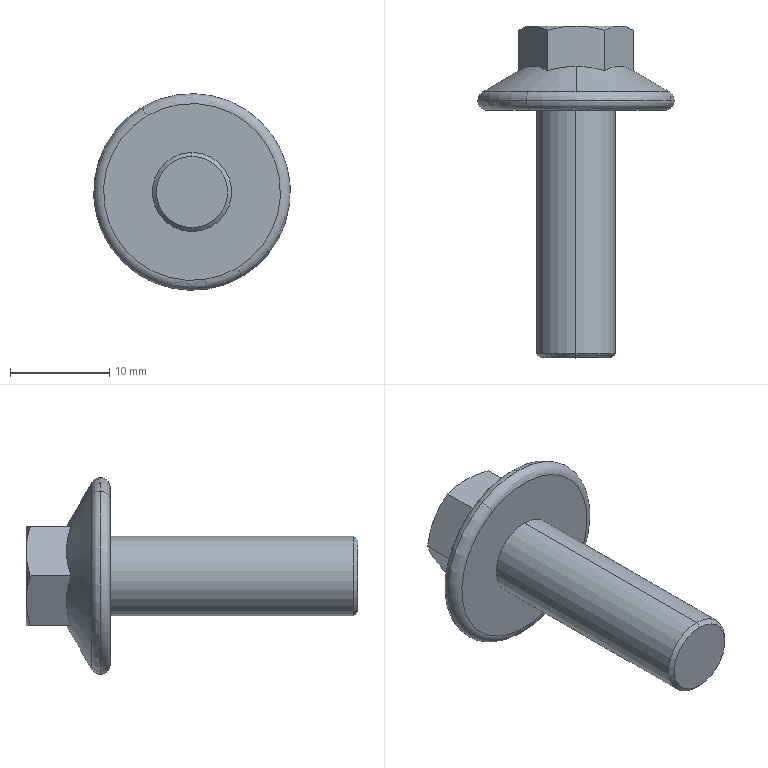Part | STEP file | VD-60063402_1_VD-SYL0380-322120 | 1 solid | 25 faces | box 19.856 x 33.5 x 19.856 mm | volume 2596 mm3 | cone 10 | plane 9 | torus 4 | cylinder 2 | commonest cylinder face diameters 8 x2
STEP:
#1=CARTESIAN_POINT('',(0.,-25.,3.6));
#2=VERTEX_POINT('',#1);
#3=CARTESIAN_POINT('',(0.,-25.,-3.6));
#4=VERTEX_POINT('',#3);
#5=CARTESIAN_POINT('',(0.,-25.,0.));
#6=DIRECTION('',(0.,-1.,0.));
#7=DIRECTION('',(0.,0.,1.));
#8=AXIS2_PLACEMENT_3D('',#5,#6,#7);
#9=CIRCLE('',#8,3.6);
#10=EDGE_CURVE('',#2,#4,#9,.T.);
#11=ORIENTED_EDGE('',*,*,#10,.F.);
#12=CARTESIAN_POINT('',(0.,-24.6,4.));
#13=VERTEX_POINT('',#12);
#14=CARTESIAN_POINT('',(0.,-24.6,4.));
#15=DIRECTION('',(0.,-0.7071,-0.7071));
#16=VECTOR('',#15,1000.);
#17=LINE('',#14,#16);
#18=EDGE_CURVE('',#13,#2,#17,.T.);
#19=ORIENTED_EDGE('',*,*,#18,.F.);
#20=CARTESIAN_POINT('',(0.,-24.6,-4.));
#21=VERTEX_POINT('',#20);
#22=CARTESIAN_POINT('',(0.,-24.6,0.));
#23=DIRECTION('',(0.,-1.,0.));
#24=DIRECTION('',(0.,0.,1.));
#25=AXIS2_PLACEMENT_3D('',#22,#23,#24);
#26=CIRCLE('',#25,4.);
#27=EDGE_CURVE('',#13,#21,#26,.T.);
#28=ORIENTED_EDGE('',*,*,#27,.T.);
#29=CARTESIAN_POINT('',(0.,-24.6,-4.));
#30=DIRECTION('',(0.,-0.7071,0.7071));
#31=VECTOR('',#30,1000.);
#32=LINE('',#29,#31);
#33=EDGE_CURVE('',#21,#4,#32,.T.);
#34=ORIENTED_EDGE('',*,*,#33,.T.);
#35=EDGE_LOOP('',(#11,#19,#28,#34));
#36=FACE_OUTER_BOUND('',#35,.T.);
#37=CARTESIAN_POINT('',(0.,-24.8,0.));
#38=DIRECTION('',(0.,1.,0.));
#39=DIRECTION('',(0.,0.,1.));
#40=AXIS2_PLACEMENT_3D('',#37,#38,#39);
#41=CONICAL_SURFACE('',#40,3.8,0.7854);
#42=ADVANCED_FACE('',(#36),#41,.T.);
#43=ORIENTED_EDGE('',*,*,#10,.T.);
#44=CARTESIAN_POINT('',(0.,-25.,0.));
#45=DIRECTION('',(0.,-1.,0.));
#46=DIRECTION('',(0.,0.,-1.));
#47=AXIS2_PLACEMENT_3D('',#44,#45,#46);
#48=CIRCLE('',#47,3.6);
#49=EDGE_CURVE('',#4,#2,#48,.T.);
#50=ORIENTED_EDGE('',*,*,#49,.T.);
#51=EDGE_LOOP('',(#43,#50));
#52=FACE_OUTER_BOUND('',#51,.T.);
#53=CARTESIAN_POINT('',(0.,-25.,0.));
#54=DIRECTION('',(0.,1.,0.));
#55=DIRECTION('',(1.,0.,0.));
#56=AXIS2_PLACEMENT_3D('',#53,#54,#55);
#57=PLANE('',#56);
#58=ADVANCED_FACE('',(#52),#57,.F.);
#59=ORIENTED_EDGE('',*,*,#33,.F.);
#60=CARTESIAN_POINT('',(0.,-24.6,0.));
#61=DIRECTION('',(0.,-1.,0.));
#62=DIRECTION('',(0.,0.,-1.));
#63=AXIS2_PLACEMENT_3D('',#60,#61,#62);
#64=CIRCLE('',#63,4.);
#65=EDGE_CURVE('',#21,#13,#64,.T.);
#66=ORIENTED_EDGE('',*,*,#65,.T.);
#67=ORIENTED_EDGE('',*,*,#18,.T.);
#68=ORIENTED_EDGE('',*,*,#49,.F.);
#69=EDGE_LOOP('',(#59,#66,#67,#68));
#70=FACE_OUTER_BOUND('',#69,.T.);
#71=CARTESIAN_POINT('',(0.,-24.8,0.));
#72=DIRECTION('',(0.,1.,0.));
#73=DIRECTION('',(0.,0.,1.));
#74=AXIS2_PLACEMENT_3D('',#71,#72,#73);
#75=CONICAL_SURFACE('',#74,3.8,0.7854);
#76=ADVANCED_FACE('',(#70),#75,.T.);
#77=CARTESIAN_POINT('',(0.,0.,-4.));
#78=VERTEX_POINT('',#77);
#79=CARTESIAN_POINT('',(0.,0.,-4.));
#80=DIRECTION('',(0.,-1.,0.));
#81=VECTOR('',#80,1000.);
#82=LINE('',#79,#81);
#83=EDGE_CURVE('',#78,#21,#82,.T.);
#84=ORIENTED_EDGE('',*,*,#83,.F.);
#85=CARTESIAN_POINT('',(0.,0.,4.));
#86=VERTEX_POINT('',#85);
#87=CARTESIAN_POINT('',(0.,0.,0.));
#88=DIRECTION('',(0.,1.,0.));
#89=DIRECTION('',(0.,0.,1.));
#90=AXIS2_PLACEMENT_3D('',#87,#88,#89);
#91=CIRCLE('',#90,4.);
#92=EDGE_CURVE('',#86,#78,#91,.T.);
#93=ORIENTED_EDGE('',*,*,#92,.F.);
#94=CARTESIAN_POINT('',(0.,0.,4.));
#95=DIRECTION('',(0.,-1.,0.));
#96=VECTOR('',#95,1000.);
#97=LINE('',#94,#96);
#98=EDGE_CURVE('',#86,#13,#97,.T.);
#99=ORIENTED_EDGE('',*,*,#98,.T.);
#100=ORIENTED_EDGE('',*,*,#65,.F.);
#101=EDGE_LOOP('',(#84,#93,#99,#100));
#102=FACE_OUTER_BOUND('',#101,.T.);
#103=CARTESIAN_POINT('',(0.,-26.25,0.));
#104=DIRECTION('',(0.,1.,0.));
#105=DIRECTION('',(0.,0.,1.));
#106=AXIS2_PLACEMENT_3D('',#103,#104,#105);
#107=CYLINDRICAL_SURFACE('',#106,4.);
#108=ADVANCED_FACE('',(#102),#107,.T.);
#109=ORIENTED_EDGE('',*,*,#27,.F.);
#110=ORIENTED_EDGE('',*,*,#98,.F.);
#111=CARTESIAN_POINT('',(0.,0.,0.));
#112=DIRECTION('',(0.,1.,0.));
#113=DIRECTION('',(0.,0.,-1.));
#114=AXIS2_PLACEMENT_3D('',#111,#112,#113);
#115=CIRCLE('',#114,4.);
#116=EDGE_CURVE('',#78,#86,#115,.T.);
#117=ORIENTED_EDGE('',*,*,#116,.F.);
#118=ORIENTED_EDGE('',*,*,#83,.T.);
#119=EDGE_LOOP('',(#109,#110,#117,#118));
#120=FACE_OUTER_BOUND('',#119,.T.);
#121=CARTESIAN_POINT('',(0.,-26.25,0.));
#122=DIRECTION('',(0.,1.,0.));
#123=DIRECTION('',(0.,0.,1.));
#124=AXIS2_PLACEMENT_3D('',#121,#122,#123);
#125=CYLINDRICAL_SURFACE('',#124,4.);
#126=ADVANCED_FACE('',(#120),#125,.T.);
#127=CARTESIAN_POINT('',(-5.038,1.,8.555));
#128=VERTEX_POINT('',#127);
#129=CARTESIAN_POINT('',(5.038,1.,-8.555));
#130=VERTEX_POINT('',#129);
#131=CARTESIAN_POINT('',(0.,1.,0.));
#132=DIRECTION('',(0.,1.,0.));
#133=DIRECTION('',(-0.5075,0.,0.8617));
#134=AXIS2_PLACEMENT_3D('',#131,#132,#133);
#135=CIRCLE('',#134,9.928);
#136=EDGE_CURVE('',#128,#130,#135,.T.);
#137=ORIENTED_EDGE('',*,*,#136,.T.);
#138=CARTESIAN_POINT('',(4.785,1.866,-8.124));
#139=VERTEX_POINT('',#138);
#140=CARTESIAN_POINT('',(4.531,1.,-7.693));
#141=DIRECTION('',(-0.8617,0.,-0.5075));
#142=DIRECTION('',(0.2537,0.866,-0.4308));
#143=AXIS2_PLACEMENT_3D('',#140,#141,#142);
#144=CIRCLE('',#143,1.);
#145=EDGE_CURVE('',#139,#130,#144,.T.);
#146=ORIENTED_EDGE('',*,*,#145,.F.);
#147=CARTESIAN_POINT('',(0.,1.866,9.428));
#148=VERTEX_POINT('',#147);
#149=CARTESIAN_POINT('',(0.,1.866,0.));
#150=DIRECTION('',(0.,-1.,0.));
#151=DIRECTION('',(0.5075,0.,-0.8617));
#152=AXIS2_PLACEMENT_3D('',#149,#150,#151);
#153=CIRCLE('',#152,9.428);
#154=EDGE_CURVE('',#139,#148,#153,.T.);
#155=ORIENTED_EDGE('',*,*,#154,.T.);
#156=CARTESIAN_POINT('',(-4.785,1.866,8.124));
#157=VERTEX_POINT('',#156);
#158=CARTESIAN_POINT('',(0.,1.866,0.));
#159=DIRECTION('',(0.,-1.,0.));
#160=DIRECTION('',(0.,0.,1.));
#161=AXIS2_PLACEMENT_3D('',#158,#159,#160);
#162=CIRCLE('',#161,9.428);
#163=EDGE_CURVE('',#148,#157,#162,.T.);
#164=ORIENTED_EDGE('',*,*,#163,.T.);
#165=CARTESIAN_POINT('',(-4.531,1.,7.693));
#166=DIRECTION('',(0.8617,0.,0.5075));
#167=DIRECTION('',(-0.2537,0.866,0.4308));
#168=AXIS2_PLACEMENT_3D('',#165,#166,#167);
#169=CIRCLE('',#168,1.);
#170=EDGE_CURVE('',#157,#128,#169,.T.);
#171=ORIENTED_EDGE('',*,*,#170,.T.);
#172=EDGE_LOOP('',(#137,#146,#155,#164,#171));
#173=FACE_OUTER_BOUND('',#172,.T.);
#174=CARTESIAN_POINT('',(0.,1.,0.));
#175=DIRECTION('',(0.,1.,0.));
#176=DIRECTION('',(0.5075,0.,-0.8617));
#177=AXIS2_PLACEMENT_3D('',#174,#175,#176);
#178=TOROIDAL_SURFACE('',#177,8.928,1.);
#179=ADVANCED_FACE('',(#173),#178,.T.);
#180=CARTESIAN_POINT('',(-4.464,0.000000001,7.732));
#181=VERTEX_POINT('',#180);
#182=CARTESIAN_POINT('',(-4.531,0.000000001,7.693));
#183=VERTEX_POINT('',#182);
#184=CARTESIAN_POINT('',(0.,0.,0.));
#185=DIRECTION('',(0.,-1.,0.));
#186=DIRECTION('',(-0.5,0.,0.866));
#187=AXIS2_PLACEMENT_3D('',#184,#185,#186);
#188=CIRCLE('',#187,8.928);
#189=EDGE_CURVE('',#181,#183,#188,.T.);
#190=ORIENTED_EDGE('',*,*,#189,.F.);
#191=CARTESIAN_POINT('',(4.531,0.000000001,-7.693));
#192=VERTEX_POINT('',#191);
#193=CARTESIAN_POINT('',(0.,0.000000001,0.));
#194=DIRECTION('',(0.,-1.,0.));
#195=DIRECTION('',(0.5075,0.,-0.8617));
#196=AXIS2_PLACEMENT_3D('',#193,#194,#195);
#197=CIRCLE('',#196,8.928);
#198=EDGE_CURVE('',#192,#181,#197,.T.);
#199=ORIENTED_EDGE('',*,*,#198,.F.);
#200=CARTESIAN_POINT('',(4.531,1.,-7.693));
#201=DIRECTION('',(-0.8617,0.,-0.5075));
#202=DIRECTION('',(0.5075,0.,-0.8617));
#203=AXIS2_PLACEMENT_3D('',#200,#201,#202);
#204=CIRCLE('',#203,1.);
#205=EDGE_CURVE('',#130,#192,#204,.T.);
#206=ORIENTED_EDGE('',*,*,#205,.F.);
#207=ORIENTED_EDGE('',*,*,#136,.F.);
#208=CARTESIAN_POINT('',(-4.531,1.,7.693));
#209=DIRECTION('',(0.8617,0.,0.5075));
#210=DIRECTION('',(-0.5075,0.,0.8617));
#211=AXIS2_PLACEMENT_3D('',#208,#209,#210);
#212=CIRCLE('',#211,1.);
#213=EDGE_CURVE('',#128,#183,#212,.T.);
#214=ORIENTED_EDGE('',*,*,#213,.T.);
#215=EDGE_LOOP('',(#190,#199,#206,#207,#214));
#216=FACE_OUTER_BOUND('',#215,.T.);
#217=CARTESIAN_POINT('',(0.,1.,0.));
#218=DIRECTION('',(0.,1.,0.));
#219=DIRECTION('',(0.5075,0.,-0.8617));
#220=AXIS2_PLACEMENT_3D('',#217,#218,#219);
#221=TOROIDAL_SURFACE('',#220,8.928,1.);
#222=ADVANCED_FACE('',(#216),#221,.T.);
#223=ORIENTED_EDGE('',*,*,#92,.T.);
#224=ORIENTED_EDGE('',*,*,#116,.T.);
#225=EDGE_LOOP('',(#223,#224));
#226=FACE_BOUND('',#225,.T.);
#227=ORIENTED_EDGE('',*,*,#189,.T.);
#228=CARTESIAN_POINT('',(4.464,0.000000001,-7.732));
#229=VERTEX_POINT('',#228);
#230=CARTESIAN_POINT('',(0.,0.000000001,0.));
#231=DIRECTION('',(0.,-1.,0.));
#232=DIRECTION('',(-0.5075,0.,0.8617));
#233=AXIS2_PLACEMENT_3D('',#230,#231,#232);
#234=CIRCLE('',#233,8.928);
#235=EDGE_CURVE('',#183,#229,#234,.T.);
#236=ORIENTED_EDGE('',*,*,#235,.T.);
#237=CARTESIAN_POINT('',(0.,0.,0.));
#238=DIRECTION('',(0.,-1.,0.));
#239=DIRECTION('',(0.5,0.,-0.866));
#240=AXIS2_PLACEMENT_3D('',#237,#238,#239);
#241=CIRCLE('',#240,8.928);
#242=EDGE_CURVE('',#229,#192,#241,.T.);
#243=ORIENTED_EDGE('',*,*,#242,.T.);
#244=ORIENTED_EDGE('',*,*,#198,.T.);
#245=EDGE_LOOP('',(#227,#236,#243,#244));
#246=FACE_OUTER_BOUND('',#245,.T.);
#247=CARTESIAN_POINT('',(0.,0.,0.));
#248=DIRECTION('',(0.,1.,0.));
#249=DIRECTION('',(1.,0.,0.));
#250=AXIS2_PLACEMENT_3D('',#247,#248,#249);
#251=PLANE('',#250);
#252=ADVANCED_FACE('',(#226,#246),#251,.F.);
#253=ORIENTED_EDGE('',*,*,#213,.F.);
#254=CARTESIAN_POINT('',(0.,1.,0.));
#255=DIRECTION('',(0.,1.,0.));
#256=DIRECTION('',(0.5075,0.,-0.8617));
#257=AXIS2_PLACEMENT_3D('',#254,#255,#256);
#258=CIRCLE('',#257,9.928);
#259=EDGE_CURVE('',#130,#128,#258,.T.);
#260=ORIENTED_EDGE('',*,*,#259,.F.);
#261=ORIENTED_EDGE('',*,*,#205,.T.);
#262=ORIENTED_EDGE('',*,*,#242,.F.);
#263=ORIENTED_EDGE('',*,*,#235,.F.);
#264=EDGE_LOOP('',(#253,#260,#261,#262,#263));
#265=FACE_OUTER_BOUND('',#264,.T.);
#266=CARTESIAN_POINT('',(0.,1.,0.));
#267=DIRECTION('',(0.,1.,0.));
#268=DIRECTION('',(-0.5075,0.,0.8617));
#269=AXIS2_PLACEMENT_3D('',#266,#267,#268);
#270=TOROIDAL_SURFACE('',#269,8.928,1.);
#271=ADVANCED_FACE('',(#265),#270,.T.);
#272=ORIENTED_EDGE('',*,*,#170,.F.);
#273=CARTESIAN_POINT('',(0.,1.866,-9.428));
#274=VERTEX_POINT('',#273);
#275=CARTESIAN_POINT('',(0.,1.866,0.));
#276=DIRECTION('',(0.,-1.,0.));
#277=DIRECTION('',(-0.5075,0.,0.8617));
#278=AXIS2_PLACEMENT_3D('',#275,#276,#277);
#279=CIRCLE('',#278,9.428);
#280=EDGE_CURVE('',#157,#274,#279,.T.);
#281=ORIENTED_EDGE('',*,*,#280,.T.);
#282=CARTESIAN_POINT('',(0.,1.866,0.));
#283=DIRECTION('',(0.,-1.,0.));
#284=DIRECTION('',(0.,0.,-1.));
#285=AXIS2_PLACEMENT_3D('',#282,#283,#284);
#286=CIRCLE('',#285,9.428);
#287=EDGE_CURVE('',#274,#139,#286,.T.);
#288=ORIENTED_EDGE('',*,*,#287,.T.);
#289=ORIENTED_EDGE('',*,*,#145,.T.);
#290=ORIENTED_EDGE('',*,*,#259,.T.);
#291=EDGE_LOOP('',(#272,#281,#288,#289,#290));
#292=FACE_OUTER_BOUND('',#291,.T.);
#293=CARTESIAN_POINT('',(0.,1.,0.));
#294=DIRECTION('',(0.,1.,0.));
#295=DIRECTION('',(-0.5075,0.,0.8617));
#296=AXIS2_PLACEMENT_3D('',#293,#294,#295);
#297=TOROIDAL_SURFACE('',#296,8.928,1.);
#298=ADVANCED_FACE('',(#292),#297,.T.);
#299=CARTESIAN_POINT('',(-2.887,8.053,-5.));
#300=VERTEX_POINT('',#299);
#301=CARTESIAN_POINT('',(-4.33,8.5,-2.5));
#302=VERTEX_POINT('',#301);
#303=CARTESIAN_POINT('',(-2.887,8.053,-5.));
#304=CARTESIAN_POINT('',(-3.013,8.126,-4.781));
#305=CARTESIAN_POINT('',(-3.136,8.19,-4.568));
#306=CARTESIAN_POINT('',(-3.318,8.273,-4.253));
#307=CARTESIAN_POINT('',(-3.378,8.299,-4.148));
#308=CARTESIAN_POINT('',(-3.468,8.334,-3.993));
#309=CARTESIAN_POINT('',(-3.498,8.345,-3.941));
#310=CARTESIAN_POINT('',(-3.558,8.366,-3.837));
#311=CARTESIAN_POINT('',(-3.587,8.375,-3.787));
#312=CARTESIAN_POINT('',(-3.861,8.462,-3.313));
#313=CARTESIAN_POINT('',(-4.092,8.5,-2.912));
#314=CARTESIAN_POINT('',(-4.33,8.5,-2.5));
#315=B_SPLINE_CURVE_WITH_KNOTS('',3,(#303,#304,#305,#306,#307,#308,#309,#310,#311,#312,#313,#314),.UNSPECIFIED.,.F.,.F.,(4,2,2,2,2,4),(0.,0.25,0.375,0.4375,0.5,1.),.UNSPECIFIED.);
#316=EDGE_CURVE('',#300,#302,#315,.T.);
#317=ORIENTED_EDGE('',*,*,#316,.T.);
#318=CARTESIAN_POINT('',(0.,8.5,-5.));
#319=VERTEX_POINT('',#318);
#320=CARTESIAN_POINT('',(0.,8.5,0.));
#321=DIRECTION('',(0.,1.,0.));
#322=DIRECTION('',(0.,0.,-1.));
#323=AXIS2_PLACEMENT_3D('',#320,#321,#322);
#324=CIRCLE('',#323,5.);
#325=EDGE_CURVE('',#319,#302,#324,.T.);
#326=ORIENTED_EDGE('',*,*,#325,.F.);
#327=CARTESIAN_POINT('',(0.,8.5,-5.));
#328=CARTESIAN_POINT('',(-0.2381,8.5,-5.));
#329=CARTESIAN_POINT('',(-0.4729,8.49,-5.));
#330=CARTESIAN_POINT('',(-0.8272,8.462,-5.));
#331=CARTESIAN_POINT('',(-0.9457,8.45,-5.));
#332=CARTESIAN_POINT('',(-1.125,8.428,-5.));
#333=CARTESIAN_POINT('',(-1.185,8.42,-5.));
#334=CARTESIAN_POINT('',(-1.305,8.403,-5.));
#335=CARTESIAN_POINT('',(-1.367,8.394,-5.));
#336=CARTESIAN_POINT('',(-1.903,8.31,-5.));
#337=CARTESIAN_POINT('',(-2.382,8.199,-5.));
#338=CARTESIAN_POINT('',(-2.887,8.053,-5.));
#339=B_SPLINE_CURVE_WITH_KNOTS('',3,(#327,#328,#329,#330,#331,#332,#333,#334,#335,#336,#337,#338),.UNSPECIFIED.,.F.,.F.,(4,2,2,2,2,4),(0.,0.25,0.375,0.4375,0.5,1.),.UNSPECIFIED.);
#340=EDGE_CURVE('',#319,#300,#339,.T.);
#341=ORIENTED_EDGE('',*,*,#340,.T.);
#342=EDGE_LOOP('',(#317,#326,#341));
#343=FACE_OUTER_BOUND('',#342,.T.);
#344=CARTESIAN_POINT('',(0.,8.277,0.));
#345=DIRECTION('',(0.,-1.,0.));
#346=DIRECTION('',(0.,0.,-1.));
#347=AXIS2_PLACEMENT_3D('',#344,#345,#346);
#348=CONICAL_SURFACE('',#347,5.387,1.047);
#349=ADVANCED_FACE('',(#343),#348,.T.);
#350=CARTESIAN_POINT('',(-5.774,8.053,0.));
#351=VERTEX_POINT('',#350);
#352=CARTESIAN_POINT('',(-4.33,8.5,-2.5));
#353=CARTESIAN_POINT('',(-4.449,8.5,-2.294));
#354=CARTESIAN_POINT('',(-4.566,8.49,-2.09));
#355=CARTESIAN_POINT('',(-4.744,8.462,-1.784));
#356=CARTESIAN_POINT('',(-4.803,8.45,-1.681));
#357=CARTESIAN_POINT('',(-4.893,8.428,-1.526));
#358=CARTESIAN_POINT('',(-4.923,8.42,-1.474));
#359=CARTESIAN_POINT('',(-4.983,8.403,-1.37));
#360=CARTESIAN_POINT('',(-5.014,8.394,-1.317));
#361=CARTESIAN_POINT('',(-5.281,8.31,-0.8521));
#362=CARTESIAN_POINT('',(-5.521,8.199,-0.4369));
#363=CARTESIAN_POINT('',(-5.774,8.053,0.));
#364=B_SPLINE_CURVE_WITH_KNOTS('',3,(#352,#353,#354,#355,#356,#357,#358,#359,#360,#361,#362,#363),.UNSPECIFIED.,.F.,.F.,(4,2,2,2,2,4),(0.,0.25,0.375,0.4375,0.5,1.),.UNSPECIFIED.);
#365=EDGE_CURVE('',#302,#351,#364,.T.);
#366=ORIENTED_EDGE('',*,*,#365,.T.);
#367=CARTESIAN_POINT('',(-4.33,8.5,2.5));
#368=VERTEX_POINT('',#367);
#369=CARTESIAN_POINT('',(-5.774,8.053,0.));
#370=CARTESIAN_POINT('',(-5.647,8.126,0.2187));
#371=CARTESIAN_POINT('',(-5.524,8.19,0.432));
#372=CARTESIAN_POINT('',(-5.342,8.273,0.7473));
#373=CARTESIAN_POINT('',(-5.282,8.299,0.8516));
#374=CARTESIAN_POINT('',(-5.192,8.334,1.007));
#375=CARTESIAN_POINT('',(-5.162,8.345,1.059));
#376=CARTESIAN_POINT('',(-5.102,8.366,1.163));
#377=CARTESIAN_POINT('',(-5.073,8.375,1.213));
#378=CARTESIAN_POINT('',(-4.8,8.462,1.687));
#379=CARTESIAN_POINT('',(-4.568,8.5,2.088));
#380=CARTESIAN_POINT('',(-4.33,8.5,2.5));
#381=B_SPLINE_CURVE_WITH_KNOTS('',3,(#369,#370,#371,#372,#373,#374,#375,#376,#377,#378,#379,#380),.UNSPECIFIED.,.F.,.F.,(4,2,2,2,2,4),(0.,0.25,0.375,0.4375,0.5,1.),.UNSPECIFIED.);
#382=EDGE_CURVE('',#351,#368,#381,.T.);
#383=ORIENTED_EDGE('',*,*,#382,.T.);
#384=CARTESIAN_POINT('',(0.,8.5,0.));
#385=DIRECTION('',(0.,1.,0.));
#386=DIRECTION('',(-0.866,0.,-0.5));
#387=AXIS2_PLACEMENT_3D('',#384,#385,#386);
#388=CIRCLE('',#387,5.);
#389=EDGE_CURVE('',#302,#368,#388,.T.);
#390=ORIENTED_EDGE('',*,*,#389,.F.);
#391=EDGE_LOOP('',(#366,#383,#390));
#392=FACE_OUTER_BOUND('',#391,.T.);
#393=CARTESIAN_POINT('',(0.,8.277,0.));
#394=DIRECTION('',(0.,-1.,0.));
#395=DIRECTION('',(0.,0.,-1.));
#396=AXIS2_PLACEMENT_3D('',#393,#394,#395);
#397=CONICAL_SURFACE('',#396,5.387,1.047);
#398=ADVANCED_FACE('',(#392),#397,.T.);
#399=CARTESIAN_POINT('',(-2.887,8.053,5.));
#400=VERTEX_POINT('',#399);
#401=CARTESIAN_POINT('',(-4.33,8.5,2.5));
#402=CARTESIAN_POINT('',(-4.211,8.5,2.706));
#403=CARTESIAN_POINT('',(-4.093,8.49,2.909));
#404=CARTESIAN_POINT('',(-3.916,8.462,3.216));
#405=CARTESIAN_POINT('',(-3.857,8.45,3.319));
#406=CARTESIAN_POINT('',(-3.768,8.428,3.474));
#407=CARTESIAN_POINT('',(-3.738,8.42,3.526));
#408=CARTESIAN_POINT('',(-3.678,8.403,3.63));
#409=CARTESIAN_POINT('',(-3.647,8.394,3.684));
#410=CARTESIAN_POINT('',(-3.379,8.31,4.148));
#411=CARTESIAN_POINT('',(-3.139,8.199,4.563));
#412=CARTESIAN_POINT('',(-2.887,8.053,5.));
#413=B_SPLINE_CURVE_WITH_KNOTS('',3,(#401,#402,#403,#404,#405,#406,#407,#408,#409,#410,#411,#412),.UNSPECIFIED.,.F.,.F.,(4,2,2,2,2,4),(0.,0.25,0.375,0.4375,0.5,1.),.UNSPECIFIED.);
#414=EDGE_CURVE('',#368,#400,#413,.T.);
#415=ORIENTED_EDGE('',*,*,#414,.T.);
#416=CARTESIAN_POINT('',(-0.000000014,8.5,5.));
#417=VERTEX_POINT('',#416);
#418=CARTESIAN_POINT('',(-2.887,8.053,5.));
#419=CARTESIAN_POINT('',(-2.634,8.126,5.));
#420=CARTESIAN_POINT('',(-2.388,8.19,5.));
#421=CARTESIAN_POINT('',(-2.024,8.273,5.));
#422=CARTESIAN_POINT('',(-1.903,8.299,5.));
#423=CARTESIAN_POINT('',(-1.723,8.334,5.));
#424=CARTESIAN_POINT('',(-1.664,8.345,5.));
#425=CARTESIAN_POINT('',(-1.544,8.366,5.));
#426=CARTESIAN_POINT('',(-1.486,8.375,5.));
#427=CARTESIAN_POINT('',(-0.9388,8.462,5.001));
#428=CARTESIAN_POINT('',(-0.4757,8.5,5.));
#429=CARTESIAN_POINT('',(-0.000000014,8.5,5.));
#430=B_SPLINE_CURVE_WITH_KNOTS('',3,(#418,#419,#420,#421,#422,#423,#424,#425,#426,#427,#428,#429),.UNSPECIFIED.,.F.,.F.,(4,2,2,2,2,4),(0.,0.25,0.375,0.4375,0.5,1.),.UNSPECIFIED.);
#431=EDGE_CURVE('',#400,#417,#430,.T.);
#432=ORIENTED_EDGE('',*,*,#431,.T.);
#433=CARTESIAN_POINT('',(0.,8.5,0.));
#434=DIRECTION('',(0.,1.,0.));
#435=DIRECTION('',(-0.866,0.,0.5));
#436=AXIS2_PLACEMENT_3D('',#433,#434,#435);
#437=CIRCLE('',#436,5.);
#438=EDGE_CURVE('',#368,#417,#437,.T.);
#439=ORIENTED_EDGE('',*,*,#438,.F.);
#440=EDGE_LOOP('',(#415,#432,#439));
#441=FACE_OUTER_BOUND('',#440,.T.);
#442=CARTESIAN_POINT('',(0.,8.277,0.));
#443=DIRECTION('',(0.,-1.,0.));
#444=DIRECTION('',(0.,0.,-1.));
#445=AXIS2_PLACEMENT_3D('',#442,#443,#444);
#446=CONICAL_SURFACE('',#445,5.387,1.047);
#447=ADVANCED_FACE('',(#441),#446,.T.);
#448=CARTESIAN_POINT('',(4.33,8.5,2.5));
#449=VERTEX_POINT('',#448);
#450=CARTESIAN_POINT('',(5.774,8.053,0.));
#451=VERTEX_POINT('',#450);
#452=CARTESIAN_POINT('',(4.33,8.5,2.5));
#453=CARTESIAN_POINT('',(4.449,8.5,2.294));
#454=CARTESIAN_POINT('',(4.566,8.49,2.09));
#455=CARTESIAN_POINT('',(4.744,8.462,1.784));
#456=CARTESIAN_POINT('',(4.803,8.45,1.681));
#457=CARTESIAN_POINT('',(4.893,8.428,1.526));
#458=CARTESIAN_POINT('',(4.923,8.42,1.474));
#459=CARTESIAN_POINT('',(4.983,8.403,1.37));
#460=CARTESIAN_POINT('',(5.014,8.394,1.317));
#461=CARTESIAN_POINT('',(5.281,8.31,0.8521));
#462=CARTESIAN_POINT('',(5.521,8.199,0.4369));
#463=CARTESIAN_POINT('',(5.774,8.053,0.));
#464=B_SPLINE_CURVE_WITH_KNOTS('',3,(#452,#453,#454,#455,#456,#457,#458,#459,#460,#461,#462,#463),.UNSPECIFIED.,.F.,.F.,(4,2,2,2,2,4),(0.,0.25,0.375,0.4375,0.5,1.),.UNSPECIFIED.);
#465=EDGE_CURVE('',#449,#451,#464,.T.);
#466=ORIENTED_EDGE('',*,*,#465,.T.);
#467=CARTESIAN_POINT('',(4.33,8.5,-2.5));
#468=VERTEX_POINT('',#467);
#469=CARTESIAN_POINT('',(5.774,8.053,0.));
#470=CARTESIAN_POINT('',(5.647,8.126,-0.2187));
#471=CARTESIAN_POINT('',(5.524,8.19,-0.432));
#472=CARTESIAN_POINT('',(5.342,8.273,-0.7473));
#473=CARTESIAN_POINT('',(5.282,8.299,-0.8516));
#474=CARTESIAN_POINT('',(5.192,8.334,-1.007));
#475=CARTESIAN_POINT('',(5.162,8.345,-1.059));
#476=CARTESIAN_POINT('',(5.102,8.366,-1.163));
#477=CARTESIAN_POINT('',(5.073,8.375,-1.213));
#478=CARTESIAN_POINT('',(4.8,8.462,-1.687));
#479=CARTESIAN_POINT('',(4.568,8.5,-2.088));
#480=CARTESIAN_POINT('',(4.33,8.5,-2.5));
#481=B_SPLINE_CURVE_WITH_KNOTS('',3,(#469,#470,#471,#472,#473,#474,#475,#476,#477,#478,#479,#480),.UNSPECIFIED.,.F.,.F.,(4,2,2,2,2,4),(0.,0.25,0.375,0.4375,0.5,1.),.UNSPECIFIED.);
#482=EDGE_CURVE('',#451,#468,#481,.T.);
#483=ORIENTED_EDGE('',*,*,#482,.T.);
#484=CARTESIAN_POINT('',(0.,8.5,0.));
#485=DIRECTION('',(0.,1.,0.));
#486=DIRECTION('',(0.866,0.,0.5));
#487=AXIS2_PLACEMENT_3D('',#484,#485,#486);
#488=CIRCLE('',#487,5.);
#489=EDGE_CURVE('',#449,#468,#488,.T.);
#490=ORIENTED_EDGE('',*,*,#489,.F.);
#491=EDGE_LOOP('',(#466,#483,#490));
#492=FACE_OUTER_BOUND('',#491,.T.);
#493=CARTESIAN_POINT('',(0.,8.277,0.));
#494=DIRECTION('',(0.,-1.,0.));
#495=DIRECTION('',(0.,0.,-1.));
#496=AXIS2_PLACEMENT_3D('',#493,#494,#495);
#497=CONICAL_SURFACE('',#496,5.387,1.047);
#498=ADVANCED_FACE('',(#492),#497,.T.);
#499=CARTESIAN_POINT('',(2.887,8.053,-5.));
#500=VERTEX_POINT('',#499);
#501=CARTESIAN_POINT('',(4.33,8.5,-2.5));
#502=CARTESIAN_POINT('',(4.211,8.5,-2.706));
#503=CARTESIAN_POINT('',(4.093,8.49,-2.909));
#504=CARTESIAN_POINT('',(3.916,8.462,-3.216));
#505=CARTESIAN_POINT('',(3.857,8.45,-3.319));
#506=CARTESIAN_POINT('',(3.768,8.428,-3.474));
#507=CARTESIAN_POINT('',(3.738,8.42,-3.526));
#508=CARTESIAN_POINT('',(3.678,8.403,-3.63));
#509=CARTESIAN_POINT('',(3.647,8.394,-3.684));
#510=CARTESIAN_POINT('',(3.379,8.31,-4.148));
#511=CARTESIAN_POINT('',(3.139,8.199,-4.563));
#512=CARTESIAN_POINT('',(2.887,8.053,-5.));
#513=B_SPLINE_CURVE_WITH_KNOTS('',3,(#501,#502,#503,#504,#505,#506,#507,#508,#509,#510,#511,#512),.UNSPECIFIED.,.F.,.F.,(4,2,2,2,2,4),(0.,0.25,0.375,0.4375,0.5,1.),.UNSPECIFIED.);
#514=EDGE_CURVE('',#468,#500,#513,.T.);
#515=ORIENTED_EDGE('',*,*,#514,.T.);
#516=CARTESIAN_POINT('',(2.887,8.053,-5.));
#517=CARTESIAN_POINT('',(2.634,8.126,-5.));
#518=CARTESIAN_POINT('',(2.388,8.19,-5.));
#519=CARTESIAN_POINT('',(2.024,8.273,-5.));
#520=CARTESIAN_POINT('',(1.903,8.299,-5.));
#521=CARTESIAN_POINT('',(1.723,8.334,-5.));
#522=CARTESIAN_POINT('',(1.664,8.345,-5.));
#523=CARTESIAN_POINT('',(1.544,8.366,-5.));
#524=CARTESIAN_POINT('',(1.486,8.375,-5.));
#525=CARTESIAN_POINT('',(0.9388,8.462,-5.001));
#526=CARTESIAN_POINT('',(0.4757,8.5,-5.));
#527=CARTESIAN_POINT('',(0.,8.5,-5.));
#528=B_SPLINE_CURVE_WITH_KNOTS('',3,(#516,#517,#518,#519,#520,#521,#522,#523,#524,#525,#526,#527),.UNSPECIFIED.,.F.,.F.,(4,2,2,2,2,4),(0.,0.25,0.375,0.4375,0.5,1.),.UNSPECIFIED.);
#529=EDGE_CURVE('',#500,#319,#528,.T.);
#530=ORIENTED_EDGE('',*,*,#529,.T.);
#531=CARTESIAN_POINT('',(0.,8.5,0.));
#532=DIRECTION('',(0.,1.,0.));
#533=DIRECTION('',(0.866,0.,-0.5));
#534=AXIS2_PLACEMENT_3D('',#531,#532,#533);
#535=CIRCLE('',#534,5.);
#536=EDGE_CURVE('',#468,#319,#535,.T.);
#537=ORIENTED_EDGE('',*,*,#536,.F.);
#538=EDGE_LOOP('',(#515,#530,#537));
#539=FACE_OUTER_BOUND('',#538,.T.);
#540=CARTESIAN_POINT('',(0.,8.277,0.));
#541=DIRECTION('',(0.,-1.,0.));
#542=DIRECTION('',(0.,0.,-1.));
#543=AXIS2_PLACEMENT_3D('',#540,#541,#542);
#544=CONICAL_SURFACE('',#543,5.387,1.047);
#545=ADVANCED_FACE('',(#539),#544,.T.);
#546=ORIENTED_EDGE('',*,*,#325,.T.);
#547=ORIENTED_EDGE('',*,*,#389,.T.);
#548=ORIENTED_EDGE('',*,*,#438,.T.);
#549=CARTESIAN_POINT('',(0.,8.5,0.));
#550=DIRECTION('',(0.,1.,0.));
#551=DIRECTION('',(-0.000000003,0.,1.));
#552=AXIS2_PLACEMENT_3D('',#549,#550,#551);
#553=CIRCLE('',#552,5.);
#554=EDGE_CURVE('',#417,#449,#553,.T.);
#555=ORIENTED_EDGE('',*,*,#554,.T.);
#556=ORIENTED_EDGE('',*,*,#489,.T.);
#557=ORIENTED_EDGE('',*,*,#536,.T.);
#558=EDGE_LOOP('',(#546,#547,#548,#555,#556,#557));
#559=FACE_OUTER_BOUND('',#558,.T.);
#560=CARTESIAN_POINT('',(0.,8.5,0.));
#561=DIRECTION('',(0.,1.,0.));
#562=DIRECTION('',(1.,0.,0.));
#563=AXIS2_PLACEMENT_3D('',#560,#561,#562);
#564=PLANE('',#563);
#565=ADVANCED_FACE('',(#559),#564,.T.);
#566=CARTESIAN_POINT('',(2.887,8.053,5.));
#567=VERTEX_POINT('',#566);
#568=CARTESIAN_POINT('',(2.887,8.053,5.));
#569=CARTESIAN_POINT('',(3.013,8.126,4.781));
#570=CARTESIAN_POINT('',(3.136,8.19,4.568));
#571=CARTESIAN_POINT('',(3.318,8.273,4.253));
#572=CARTESIAN_POINT('',(3.378,8.299,4.148));
#573=CARTESIAN_POINT('',(3.468,8.334,3.993));
#574=CARTESIAN_POINT('',(3.498,8.345,3.941));
#575=CARTESIAN_POINT('',(3.558,8.366,3.837));
#576=CARTESIAN_POINT('',(3.587,8.375,3.787));
#577=CARTESIAN_POINT('',(3.861,8.462,3.313));
#578=CARTESIAN_POINT('',(4.092,8.5,2.912));
#579=CARTESIAN_POINT('',(4.33,8.5,2.5));
#580=B_SPLINE_CURVE_WITH_KNOTS('',3,(#568,#569,#570,#571,#572,#573,#574,#575,#576,#577,#578,#579),.UNSPECIFIED.,.F.,.F.,(4,2,2,2,2,4),(0.,0.25,0.375,0.4375,0.5,1.),.UNSPECIFIED.);
#581=EDGE_CURVE('',#567,#449,#580,.T.);
#582=ORIENTED_EDGE('',*,*,#581,.T.);
#583=ORIENTED_EDGE('',*,*,#554,.F.);
#584=CARTESIAN_POINT('',(-0.000000014,8.5,5.));
#585=CARTESIAN_POINT('',(0.2381,8.5,5.));
#586=CARTESIAN_POINT('',(0.4729,8.49,5.));
#587=CARTESIAN_POINT('',(0.8272,8.462,5.));
#588=CARTESIAN_POINT('',(0.9457,8.45,5.));
#589=CARTESIAN_POINT('',(1.125,8.428,5.));
#590=CARTESIAN_POINT('',(1.185,8.42,5.));
#591=CARTESIAN_POINT('',(1.305,8.403,5.));
#592=CARTESIAN_POINT('',(1.367,8.394,5.));
#593=CARTESIAN_POINT('',(1.903,8.31,5.));
#594=CARTESIAN_POINT('',(2.382,8.199,5.));
#595=CARTESIAN_POINT('',(2.887,8.053,5.));
#596=B_SPLINE_CURVE_WITH_KNOTS('',3,(#584,#585,#586,#587,#588,#589,#590,#591,#592,#593,#594,#595),.UNSPECIFIED.,.F.,.F.,(4,2,2,2,2,4),(0.,0.25,0.375,0.4375,0.5,1.),.UNSPECIFIED.);
#597=EDGE_CURVE('',#417,#567,#596,.T.);
#598=ORIENTED_EDGE('',*,*,#597,.T.);
#599=EDGE_LOOP('',(#582,#583,#598));
#600=FACE_OUTER_BOUND('',#599,.T.);
#601=CARTESIAN_POINT('',(0.,8.277,0.));
#602=DIRECTION('',(0.,-1.,0.));
#603=DIRECTION('',(0.,0.,-1.));
#604=AXIS2_PLACEMENT_3D('',#601,#602,#603);
#605=CONICAL_SURFACE('',#604,5.387,1.047);
#606=ADVANCED_FACE('',(#600),#605,.T.);
#607=CARTESIAN_POINT('',(5.774,3.976,-0.00000001));
#608=VERTEX_POINT('',#607);
#609=CARTESIAN_POINT('',(2.887,3.976,5.));
#610=VERTEX_POINT('',#609);
#611=CARTESIAN_POINT('',(5.774,3.976,-0.00000001));
#612=CARTESIAN_POINT('',(5.65,4.047,0.2142));
#613=CARTESIAN_POINT('',(5.529,4.11,0.4235));
#614=CARTESIAN_POINT('',(5.35,4.192,0.7331));
#615=CARTESIAN_POINT('',(5.291,4.217,0.8355));
#616=CARTESIAN_POINT('',(5.203,4.252,0.9886));
#617=CARTESIAN_POINT('',(5.159,4.269,1.065));
#618=CARTESIAN_POINT('',(5.115,4.284,1.141));
#619=CARTESIAN_POINT('',(5.085,4.294,1.192));
#620=CARTESIAN_POINT('',(5.071,4.298,1.216));
#621=CARTESIAN_POINT('',(4.809,4.383,1.671));
#622=CARTESIAN_POINT('',(4.574,4.423,2.078));
#623=CARTESIAN_POINT('',(4.209,4.423,2.71));
#624=CARTESIAN_POINT('',(4.089,4.413,2.917));
#625=CARTESIAN_POINT('',(3.908,4.383,3.23));
#626=CARTESIAN_POINT('',(3.848,4.371,3.334));
#627=CARTESIAN_POINT('',(3.757,4.348,3.492));
#628=CARTESIAN_POINT('',(3.711,4.336,3.571));
#629=CARTESIAN_POINT('',(3.665,4.322,3.651));
#630=CARTESIAN_POINT('',(3.635,4.313,3.704));
#631=CARTESIAN_POINT('',(3.619,4.308,3.732));
#632=CARTESIAN_POINT('',(3.37,4.228,4.163));
#633=CARTESIAN_POINT('',(3.134,4.119,4.572));
#634=CARTESIAN_POINT('',(2.887,3.976,5.));
#635=B_SPLINE_CURVE_WITH_KNOTS('',3,(#611,#612,#613,#614,#615,#616,#617,#618,#619,#620,#621,#622,#623,#624,#625,#626,#627,#628,#629,#630,#631,#632,#633,#634),.UNSPECIFIED.,.F.,.F.,(4,2,2,1,2,2,2,2,2,1,2,2,4),(0.,0.125,0.1875,0.2187,0.2344,0.25,0.5,0.625,0.6875,0.7187,0.7344,0.75,1.),.UNSPECIFIED.);
#636=EDGE_CURVE('',#608,#610,#635,.T.);
#637=ORIENTED_EDGE('',*,*,#636,.F.);
#638=CARTESIAN_POINT('',(5.774,8.053,0.));
#639=DIRECTION('',(0.000000001,-1.,-0.000000002));
#640=VECTOR('',#639,1000.);
#641=LINE('',#638,#640);
#642=EDGE_CURVE('',#451,#608,#641,.T.);
#643=ORIENTED_EDGE('',*,*,#642,.F.);
#644=ORIENTED_EDGE('',*,*,#465,.F.);
#645=ORIENTED_EDGE('',*,*,#581,.F.);
#646=CARTESIAN_POINT('',(2.887,8.053,5.));
#647=DIRECTION('',(0.000000003,-1.,0.));
#648=VECTOR('',#647,1000.);
#649=LINE('',#646,#648);
#650=EDGE_CURVE('',#567,#610,#649,.T.);
#651=ORIENTED_EDGE('',*,*,#650,.T.);
#652=EDGE_LOOP('',(#637,#643,#644,#645,#651));
#653=FACE_OUTER_BOUND('',#652,.T.);
#654=CARTESIAN_POINT('',(2.887,0.,5.));
#655=DIRECTION('',(0.866,0.,0.5));
#656=DIRECTION('',(0.,-1.,0.));
#657=AXIS2_PLACEMENT_3D('',#654,#655,#656);
#658=PLANE('',#657);
#659=ADVANCED_FACE('',(#653),#658,.T.);
#660=CARTESIAN_POINT('',(2.887,3.976,-5.));
#661=VERTEX_POINT('',#660);
#662=CARTESIAN_POINT('',(2.887,3.976,-5.));
#663=CARTESIAN_POINT('',(3.01,4.047,-4.786));
#664=CARTESIAN_POINT('',(3.131,4.11,-4.576));
#665=CARTESIAN_POINT('',(3.31,4.192,-4.267));
#666=CARTESIAN_POINT('',(3.369,4.217,-4.164));
#667=CARTESIAN_POINT('',(3.457,4.252,-4.011));
#668=CARTESIAN_POINT('',(3.502,4.269,-3.935));
#669=CARTESIAN_POINT('',(3.546,4.284,-3.859));
#670=CARTESIAN_POINT('',(3.575,4.294,-3.808));
#671=CARTESIAN_POINT('',(3.589,4.298,-3.784));
#672=CARTESIAN_POINT('',(3.851,4.383,-3.329));
#673=CARTESIAN_POINT('',(4.086,4.423,-2.922));
#674=CARTESIAN_POINT('',(4.451,4.423,-2.29));
#675=CARTESIAN_POINT('',(4.571,4.413,-2.082));
#676=CARTESIAN_POINT('',(4.751,4.383,-1.77));
#677=CARTESIAN_POINT('',(4.812,4.371,-1.665));
#678=CARTESIAN_POINT('',(4.903,4.348,-1.508));
#679=CARTESIAN_POINT('',(4.949,4.336,-1.429));
#680=CARTESIAN_POINT('',(4.995,4.322,-1.349));
#681=CARTESIAN_POINT('',(5.025,4.313,-1.296));
#682=CARTESIAN_POINT('',(5.042,4.308,-1.267));
#683=CARTESIAN_POINT('',(5.29,4.228,-0.8365));
#684=CARTESIAN_POINT('',(5.526,4.119,-0.4284));
#685=CARTESIAN_POINT('',(5.774,3.976,-0.00000001));
#686=B_SPLINE_CURVE_WITH_KNOTS('',3,(#662,#663,#664,#665,#666,#667,#668,#669,#670,#671,#672,#673,#674,#675,#676,#677,#678,#679,#680,#681,#682,#683,#684,#685),.UNSPECIFIED.,.F.,.F.,(4,2,2,1,2,2,2,2,2,1,2,2,4),(0.,0.125,0.1875,0.2188,0.2344,0.25,0.5,0.625,0.6875,0.7188,0.7344,0.75,1.),.UNSPECIFIED.);
#687=EDGE_CURVE('',#661,#608,#686,.T.);
#688=ORIENTED_EDGE('',*,*,#687,.F.);
#689=CARTESIAN_POINT('',(2.887,3.976,-5.));
#690=DIRECTION('',(0.,1.,0.));
#691=VECTOR('',#690,1000.);
#692=LINE('',#689,#691);
#693=EDGE_CURVE('',#661,#500,#692,.T.);
#694=ORIENTED_EDGE('',*,*,#693,.T.);
#695=ORIENTED_EDGE('',*,*,#514,.F.);
#696=ORIENTED_EDGE('',*,*,#482,.F.);
#697=ORIENTED_EDGE('',*,*,#642,.T.);
#698=EDGE_LOOP('',(#688,#694,#695,#696,#697));
#699=FACE_OUTER_BOUND('',#698,.T.);
#700=CARTESIAN_POINT('',(5.774,0.,0.));
#701=DIRECTION('',(0.866,0.,-0.5));
#702=DIRECTION('',(0.,-1.,0.));
#703=AXIS2_PLACEMENT_3D('',#700,#701,#702);
#704=PLANE('',#703);
#705=ADVANCED_FACE('',(#699),#704,.T.);
#706=CARTESIAN_POINT('',(0.,4.423,-5.));
#707=VERTEX_POINT('',#706);
#708=CARTESIAN_POINT('',(0.,4.423,-5.));
#709=CARTESIAN_POINT('',(0.2387,4.423,-5.));
#710=CARTESIAN_POINT('',(0.4739,4.413,-5.));
#711=CARTESIAN_POINT('',(0.8282,4.384,-5.));
#712=CARTESIAN_POINT('',(0.9465,4.372,-5.));
#713=CARTESIAN_POINT('',(1.185,4.343,-5.));
#714=CARTESIAN_POINT('',(1.307,4.326,-5.));
#715=CARTESIAN_POINT('',(1.903,4.232,-5.));
#716=CARTESIAN_POINT('',(2.383,4.122,-5.));
#717=CARTESIAN_POINT('',(2.887,3.976,-5.));
#718=B_SPLINE_CURVE_WITH_KNOTS('',3,(#708,#709,#710,#711,#712,#713,#714,#715,#716,#717),.UNSPECIFIED.,.F.,.F.,(4,2,2,2,4),(0.,0.25,0.375,0.5,1.),.UNSPECIFIED.);
#719=EDGE_CURVE('',#707,#661,#718,.T.);
#720=ORIENTED_EDGE('',*,*,#719,.F.);
#721=CARTESIAN_POINT('',(-2.887,3.976,-5.));
#722=VERTEX_POINT('',#721);
#723=CARTESIAN_POINT('',(-2.887,3.976,-5.));
#724=CARTESIAN_POINT('',(-2.635,4.049,-5.));
#725=CARTESIAN_POINT('',(-2.389,4.113,-5.));
#726=CARTESIAN_POINT('',(-2.026,4.195,-5.));
#727=CARTESIAN_POINT('',(-1.906,4.221,-5.));
#728=CARTESIAN_POINT('',(-1.727,4.256,-5.));
#729=CARTESIAN_POINT('',(-1.667,4.267,-5.));
#730=CARTESIAN_POINT('',(-1.548,4.288,-5.));
#731=CARTESIAN_POINT('',(-1.489,4.297,-5.));
#732=CARTESIAN_POINT('',(-0.9421,4.384,-5.));
#733=CARTESIAN_POINT('',(-0.4778,4.423,-5.));
#734=CARTESIAN_POINT('',(0.,4.423,-5.));
#735=B_SPLINE_CURVE_WITH_KNOTS('',3,(#723,#724,#725,#726,#727,#728,#729,#730,#731,#732,#733,#734),.UNSPECIFIED.,.F.,.F.,(4,2,2,2,2,4),(0.,0.25,0.375,0.4375,0.5,1.),.UNSPECIFIED.);
#736=EDGE_CURVE('',#722,#707,#735,.T.);
#737=ORIENTED_EDGE('',*,*,#736,.F.);
#738=CARTESIAN_POINT('',(-2.887,8.053,-5.));
#739=DIRECTION('',(-0.000000003,-1.,0.));
#740=VECTOR('',#739,1000.);
#741=LINE('',#738,#740);
#742=EDGE_CURVE('',#300,#722,#741,.T.);
#743=ORIENTED_EDGE('',*,*,#742,.F.);
#744=ORIENTED_EDGE('',*,*,#340,.F.);
#745=ORIENTED_EDGE('',*,*,#529,.F.);
#746=ORIENTED_EDGE('',*,*,#693,.F.);
#747=EDGE_LOOP('',(#720,#737,#743,#744,#745,#746));
#748=FACE_OUTER_BOUND('',#747,.T.);
#749=CARTESIAN_POINT('',(2.887,0.,-5.));
#750=DIRECTION('',(0.,0.,-1.));
#751=DIRECTION('',(0.,-1.,0.));
#752=AXIS2_PLACEMENT_3D('',#749,#750,#751);
#753=PLANE('',#752);
#754=ADVANCED_FACE('',(#748),#753,.T.);
#755=CARTESIAN_POINT('',(-5.774,3.976,0.00000001));
#756=VERTEX_POINT('',#755);
#757=CARTESIAN_POINT('',(-5.774,3.976,0.00000001));
#758=CARTESIAN_POINT('',(-5.65,4.047,-0.2142));
#759=CARTESIAN_POINT('',(-5.529,4.11,-0.4235));
#760=CARTESIAN_POINT('',(-5.35,4.192,-0.7331));
#761=CARTESIAN_POINT('',(-5.291,4.217,-0.8355));
#762=CARTESIAN_POINT('',(-5.203,4.252,-0.9886));
#763=CARTESIAN_POINT('',(-5.159,4.269,-1.065));
#764=CARTESIAN_POINT('',(-5.115,4.284,-1.141));
#765=CARTESIAN_POINT('',(-5.085,4.294,-1.192));
#766=CARTESIAN_POINT('',(-5.071,4.298,-1.216));
#767=CARTESIAN_POINT('',(-4.809,4.383,-1.671));
#768=CARTESIAN_POINT('',(-4.574,4.423,-2.078));
#769=CARTESIAN_POINT('',(-4.209,4.423,-2.71));
#770=CARTESIAN_POINT('',(-4.089,4.413,-2.917));
#771=CARTESIAN_POINT('',(-3.908,4.383,-3.23));
#772=CARTESIAN_POINT('',(-3.848,4.371,-3.334));
#773=CARTESIAN_POINT('',(-3.757,4.348,-3.492));
#774=CARTESIAN_POINT('',(-3.711,4.336,-3.571));
#775=CARTESIAN_POINT('',(-3.665,4.322,-3.651));
#776=CARTESIAN_POINT('',(-3.635,4.313,-3.704));
#777=CARTESIAN_POINT('',(-3.619,4.308,-3.732));
#778=CARTESIAN_POINT('',(-3.37,4.228,-4.163));
#779=CARTESIAN_POINT('',(-3.134,4.119,-4.572));
#780=CARTESIAN_POINT('',(-2.887,3.976,-5.));
#781=B_SPLINE_CURVE_WITH_KNOTS('',3,(#757,#758,#759,#760,#761,#762,#763,#764,#765,#766,#767,#768,#769,#770,#771,#772,#773,#774,#775,#776,#777,#778,#779,#780),.UNSPECIFIED.,.F.,.F.,(4,2,2,1,2,2,2,2,2,1,2,2,4),(0.,0.125,0.1875,0.2187,0.2344,0.25,0.5,0.625,0.6875,0.7187,0.7344,0.75,1.),.UNSPECIFIED.);
#782=EDGE_CURVE('',#756,#722,#781,.T.);
#783=ORIENTED_EDGE('',*,*,#782,.F.);
#784=CARTESIAN_POINT('',(-5.774,8.053,0.));
#785=DIRECTION('',(-0.000000001,-1.,0.000000002));
#786=VECTOR('',#785,1000.);
#787=LINE('',#784,#786);
#788=EDGE_CURVE('',#351,#756,#787,.T.);
#789=ORIENTED_EDGE('',*,*,#788,.F.);
#790=ORIENTED_EDGE('',*,*,#365,.F.);
#791=ORIENTED_EDGE('',*,*,#316,.F.);
#792=ORIENTED_EDGE('',*,*,#742,.T.);
#793=EDGE_LOOP('',(#783,#789,#790,#791,#792));
#794=FACE_OUTER_BOUND('',#793,.T.);
#795=CARTESIAN_POINT('',(-2.887,0.,-5.));
#796=DIRECTION('',(-0.866,0.,-0.5));
#797=DIRECTION('',(-0.5,0.,0.866));
#798=AXIS2_PLACEMENT_3D('',#795,#796,#797);
#799=PLANE('',#798);
#800=ADVANCED_FACE('',(#794),#799,.T.);
#801=CARTESIAN_POINT('',(-2.887,3.976,5.));
#802=VERTEX_POINT('',#801);
#803=CARTESIAN_POINT('',(-2.887,3.976,5.));
#804=CARTESIAN_POINT('',(-3.01,4.047,4.786));
#805=CARTESIAN_POINT('',(-3.131,4.11,4.576));
#806=CARTESIAN_POINT('',(-3.31,4.192,4.267));
#807=CARTESIAN_POINT('',(-3.369,4.217,4.164));
#808=CARTESIAN_POINT('',(-3.457,4.252,4.011));
#809=CARTESIAN_POINT('',(-3.502,4.269,3.935));
#810=CARTESIAN_POINT('',(-3.546,4.284,3.859));
#811=CARTESIAN_POINT('',(-3.575,4.294,3.808));
#812=CARTESIAN_POINT('',(-3.589,4.298,3.784));
#813=CARTESIAN_POINT('',(-3.851,4.383,3.329));
#814=CARTESIAN_POINT('',(-4.086,4.423,2.922));
#815=CARTESIAN_POINT('',(-4.451,4.423,2.29));
#816=CARTESIAN_POINT('',(-4.571,4.413,2.082));
#817=CARTESIAN_POINT('',(-4.751,4.383,1.77));
#818=CARTESIAN_POINT('',(-4.812,4.371,1.665));
#819=CARTESIAN_POINT('',(-4.903,4.348,1.508));
#820=CARTESIAN_POINT('',(-4.949,4.336,1.429));
#821=CARTESIAN_POINT('',(-4.995,4.322,1.349));
#822=CARTESIAN_POINT('',(-5.025,4.313,1.296));
#823=CARTESIAN_POINT('',(-5.042,4.308,1.267));
#824=CARTESIAN_POINT('',(-5.29,4.228,0.8365));
#825=CARTESIAN_POINT('',(-5.526,4.119,0.4284));
#826=CARTESIAN_POINT('',(-5.774,3.976,0.00000001));
#827=B_SPLINE_CURVE_WITH_KNOTS('',3,(#803,#804,#805,#806,#807,#808,#809,#810,#811,#812,#813,#814,#815,#816,#817,#818,#819,#820,#821,#822,#823,#824,#825,#826),.UNSPECIFIED.,.F.,.F.,(4,2,2,1,2,2,2,2,2,1,2,2,4),(0.,0.125,0.1875,0.2188,0.2344,0.25,0.5,0.625,0.6875,0.7188,0.7344,0.75,1.),.UNSPECIFIED.);
#828=EDGE_CURVE('',#802,#756,#827,.T.);
#829=ORIENTED_EDGE('',*,*,#828,.F.);
#830=CARTESIAN_POINT('',(-2.887,8.053,5.));
#831=DIRECTION('',(0.,-1.,0.));
#832=VECTOR('',#831,1000.);
#833=LINE('',#830,#832);
#834=EDGE_CURVE('',#400,#802,#833,.T.);
#835=ORIENTED_EDGE('',*,*,#834,.F.);
#836=ORIENTED_EDGE('',*,*,#414,.F.);
#837=ORIENTED_EDGE('',*,*,#382,.F.);
#838=ORIENTED_EDGE('',*,*,#788,.T.);
#839=EDGE_LOOP('',(#829,#835,#836,#837,#838));
#840=FACE_OUTER_BOUND('',#839,.T.);
#841=CARTESIAN_POINT('',(-5.774,0.,0.));
#842=DIRECTION('',(-0.866,0.,0.5));
#843=DIRECTION('',(0.,1.,0.));
#844=AXIS2_PLACEMENT_3D('',#841,#842,#843);
#845=PLANE('',#844);
#846=ADVANCED_FACE('',(#840),#845,.T.);
#847=CARTESIAN_POINT('',(0.,4.423,5.));
#848=VERTEX_POINT('',#847);
#849=CARTESIAN_POINT('',(0.,4.423,5.));
#850=CARTESIAN_POINT('',(-0.2387,4.423,5.));
#851=CARTESIAN_POINT('',(-0.4739,4.413,5.));
#852=CARTESIAN_POINT('',(-0.8282,4.384,5.));
#853=CARTESIAN_POINT('',(-0.9465,4.372,5.));
#854=CARTESIAN_POINT('',(-1.185,4.343,5.));
#855=CARTESIAN_POINT('',(-1.307,4.326,5.));
#856=CARTESIAN_POINT('',(-1.903,4.232,5.));
#857=CARTESIAN_POINT('',(-2.383,4.122,5.));
#858=CARTESIAN_POINT('',(-2.887,3.976,5.));
#859=B_SPLINE_CURVE_WITH_KNOTS('',3,(#849,#850,#851,#852,#853,#854,#855,#856,#857,#858),.UNSPECIFIED.,.F.,.F.,(4,2,2,2,4),(0.,0.25,0.375,0.5,1.),.UNSPECIFIED.);
#860=EDGE_CURVE('',#848,#802,#859,.T.);
#861=ORIENTED_EDGE('',*,*,#860,.F.);
#862=CARTESIAN_POINT('',(2.887,3.976,5.));
#863=CARTESIAN_POINT('',(2.635,4.049,5.));
#864=CARTESIAN_POINT('',(2.389,4.113,5.));
#865=CARTESIAN_POINT('',(2.026,4.195,5.));
#866=CARTESIAN_POINT('',(1.906,4.221,5.));
#867=CARTESIAN_POINT('',(1.727,4.256,5.));
#868=CARTESIAN_POINT('',(1.667,4.267,5.));
#869=CARTESIAN_POINT('',(1.548,4.288,5.));
#870=CARTESIAN_POINT('',(1.489,4.297,5.));
#871=CARTESIAN_POINT('',(0.9421,4.384,5.));
#872=CARTESIAN_POINT('',(0.4778,4.423,5.));
#873=CARTESIAN_POINT('',(0.,4.423,5.));
#874=B_SPLINE_CURVE_WITH_KNOTS('',3,(#862,#863,#864,#865,#866,#867,#868,#869,#870,#871,#872,#873),.UNSPECIFIED.,.F.,.F.,(4,2,2,2,2,4),(0.,0.25,0.375,0.4375,0.5,1.),.UNSPECIFIED.);
#875=EDGE_CURVE('',#610,#848,#874,.T.);
#876=ORIENTED_EDGE('',*,*,#875,.F.);
#877=ORIENTED_EDGE('',*,*,#650,.F.);
#878=ORIENTED_EDGE('',*,*,#597,.F.);
#879=ORIENTED_EDGE('',*,*,#431,.F.);
#880=ORIENTED_EDGE('',*,*,#834,.T.);
#881=EDGE_LOOP('',(#861,#876,#877,#878,#879,#880));
#882=FACE_OUTER_BOUND('',#881,.T.);
#883=CARTESIAN_POINT('',(-2.887,0.,5.));
#884=DIRECTION('',(0.,0.,1.));
#885=DIRECTION('',(1.,0.,0.));
#886=AXIS2_PLACEMENT_3D('',#883,#884,#885);
#887=PLANE('',#886);
#888=ADVANCED_FACE('',(#882),#887,.T.);
#889=CARTESIAN_POINT('',(0.,1.866,9.428));
#890=DIRECTION('',(0.,0.5,-0.866));
#891=VECTOR('',#890,1000.);
#892=LINE('',#889,#891);
#893=EDGE_CURVE('',#148,#848,#892,.T.);
#894=ORIENTED_EDGE('',*,*,#893,.F.);
#895=ORIENTED_EDGE('',*,*,#154,.F.);
#896=ORIENTED_EDGE('',*,*,#287,.F.);
#897=CARTESIAN_POINT('',(0.,1.866,-9.428));
#898=DIRECTION('',(0.,0.5,0.866));
#899=VECTOR('',#898,1000.);
#900=LINE('',#897,#899);
#901=EDGE_CURVE('',#274,#707,#900,.T.);
#902=ORIENTED_EDGE('',*,*,#901,.T.);
#903=ORIENTED_EDGE('',*,*,#719,.T.);
#904=ORIENTED_EDGE('',*,*,#687,.T.);
#905=ORIENTED_EDGE('',*,*,#636,.T.);
#906=ORIENTED_EDGE('',*,*,#875,.T.);
#907=EDGE_LOOP('',(#894,#895,#896,#902,#903,#904,#905,#906));
#908=FACE_OUTER_BOUND('',#907,.T.);
#909=CARTESIAN_POINT('',(0.,3.146,0.));
#910=DIRECTION('',(0.,-1.,0.));
#911=DIRECTION('',(0.,0.,-1.));
#912=AXIS2_PLACEMENT_3D('',#909,#910,#911);
#913=CONICAL_SURFACE('',#912,7.212,1.047);
#914=ADVANCED_FACE('',(#908),#913,.T.);
#915=ORIENTED_EDGE('',*,*,#860,.T.);
#916=ORIENTED_EDGE('',*,*,#828,.T.);
#917=ORIENTED_EDGE('',*,*,#782,.T.);
#918=ORIENTED_EDGE('',*,*,#736,.T.);
#919=ORIENTED_EDGE('',*,*,#901,.F.);
#920=ORIENTED_EDGE('',*,*,#280,.F.);
#921=ORIENTED_EDGE('',*,*,#163,.F.);
#922=ORIENTED_EDGE('',*,*,#893,.T.);
#923=EDGE_LOOP('',(#915,#916,#917,#918,#919,#920,#921,#922));
#924=FACE_OUTER_BOUND('',#923,.T.);
#925=CARTESIAN_POINT('',(0.,3.146,0.));
#926=DIRECTION('',(0.,-1.,0.));
#927=DIRECTION('',(0.,0.,-1.));
#928=AXIS2_PLACEMENT_3D('',#925,#926,#927);
#929=CONICAL_SURFACE('',#928,7.212,1.047);
#930=ADVANCED_FACE('',(#924),#929,.T.);
#931=CLOSED_SHELL('',(#42,#58,#76,#108,#126,#179,#222,#252,#271,#298,#349,#398,#447,#498,#545,#565,#606,#659,#705,#754,#800,#846,#888,#914,#930));
#932=MANIFOLD_SOLID_BREP('',#931);
#933=CARTESIAN_POINT('',(0.,0.,0.));
#934=DIRECTION('',(0.,0.,1.));
#935=DIRECTION('',(1.,0.,0.));
#936=AXIS2_PLACEMENT_3D('',#933,#934,#935);
#937=(LENGTH_UNIT()NAMED_UNIT(*)SI_UNIT(.MILLI.,.METRE.));
#938=UNCERTAINTY_MEASURE_WITH_UNIT(LENGTH_MEASURE(0.00001),#937,'','');
#939=(NAMED_UNIT(*)PLANE_ANGLE_UNIT()SI_UNIT($,.RADIAN.));
#940=(NAMED_UNIT(*)SI_UNIT($,.STERADIAN.)SOLID_ANGLE_UNIT());
#941=(GEOMETRIC_REPRESENTATION_CONTEXT(3)GLOBAL_UNCERTAINTY_ASSIGNED_CONTEXT((#938))GLOBAL_UNIT_ASSIGNED_CONTEXT((#937,#939,#940))REPRESENTATION_CONTEXT('',''));
#942=ADVANCED_BREP_SHAPE_REPRESENTATION('',(#932,#936),#941);